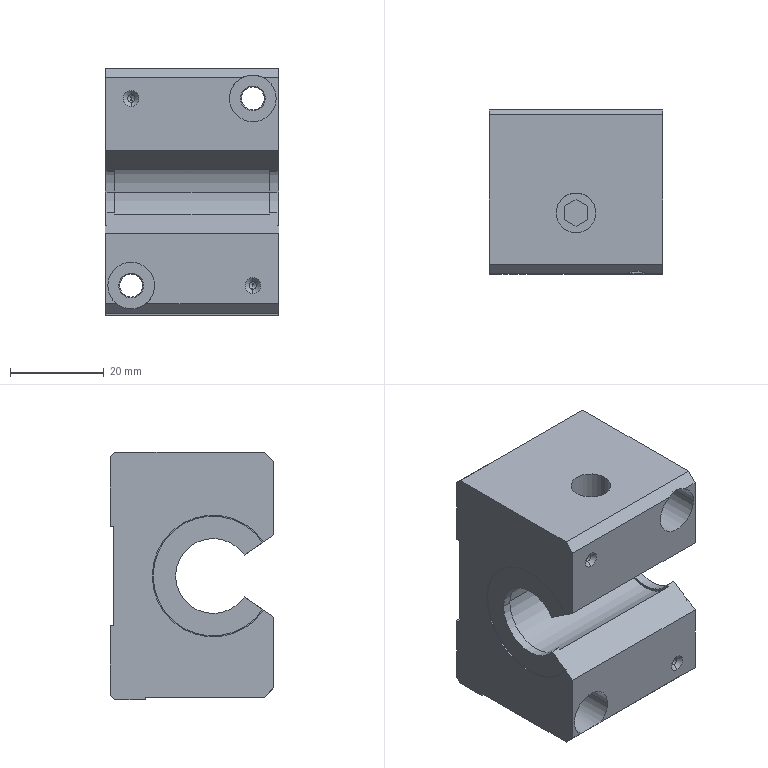Part | STEP file | b92-gnkso-16-ppas | 1 solid | 88 faces | box 37 x 35 x 53 mm | volume 52576 mm3 | plane 38 | cylinder 34 | cone 16 | commonest cylinder face diameters 1.6 x4 4.917 x4 5.3 x4 10 x4 16 x4 25.6 x4